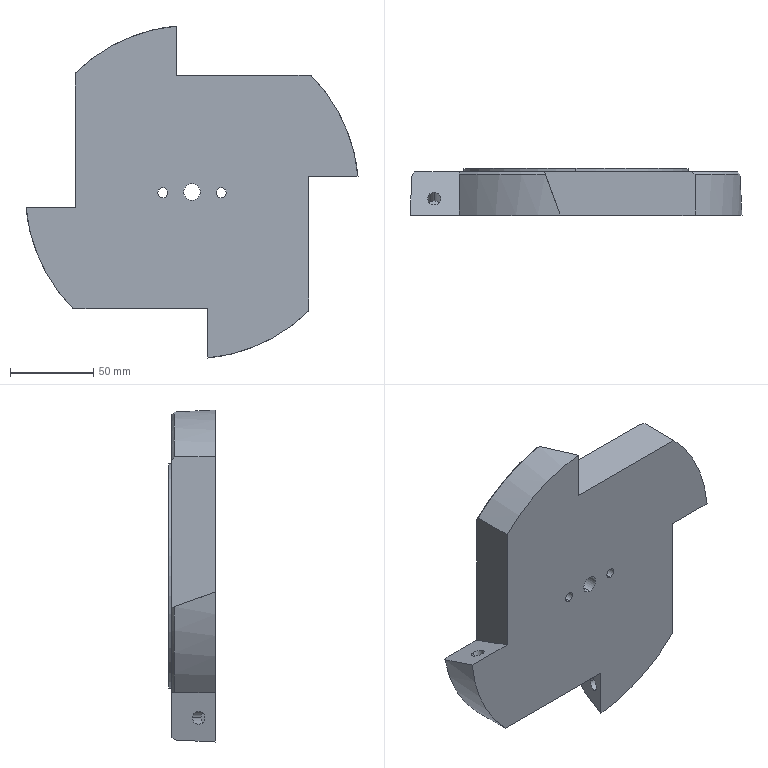Part | STEP file | Vibration plate 3-08_default | 1 solid | 45 faces | box 199.095 x 28 x 199.095 mm | volume 629211 mm3 | cylinder 24 | plane 17 | cone 4 | commonest cylinder face diameters 8 x8 6 x4 200 x4 10 x2 60 x2 105 x2